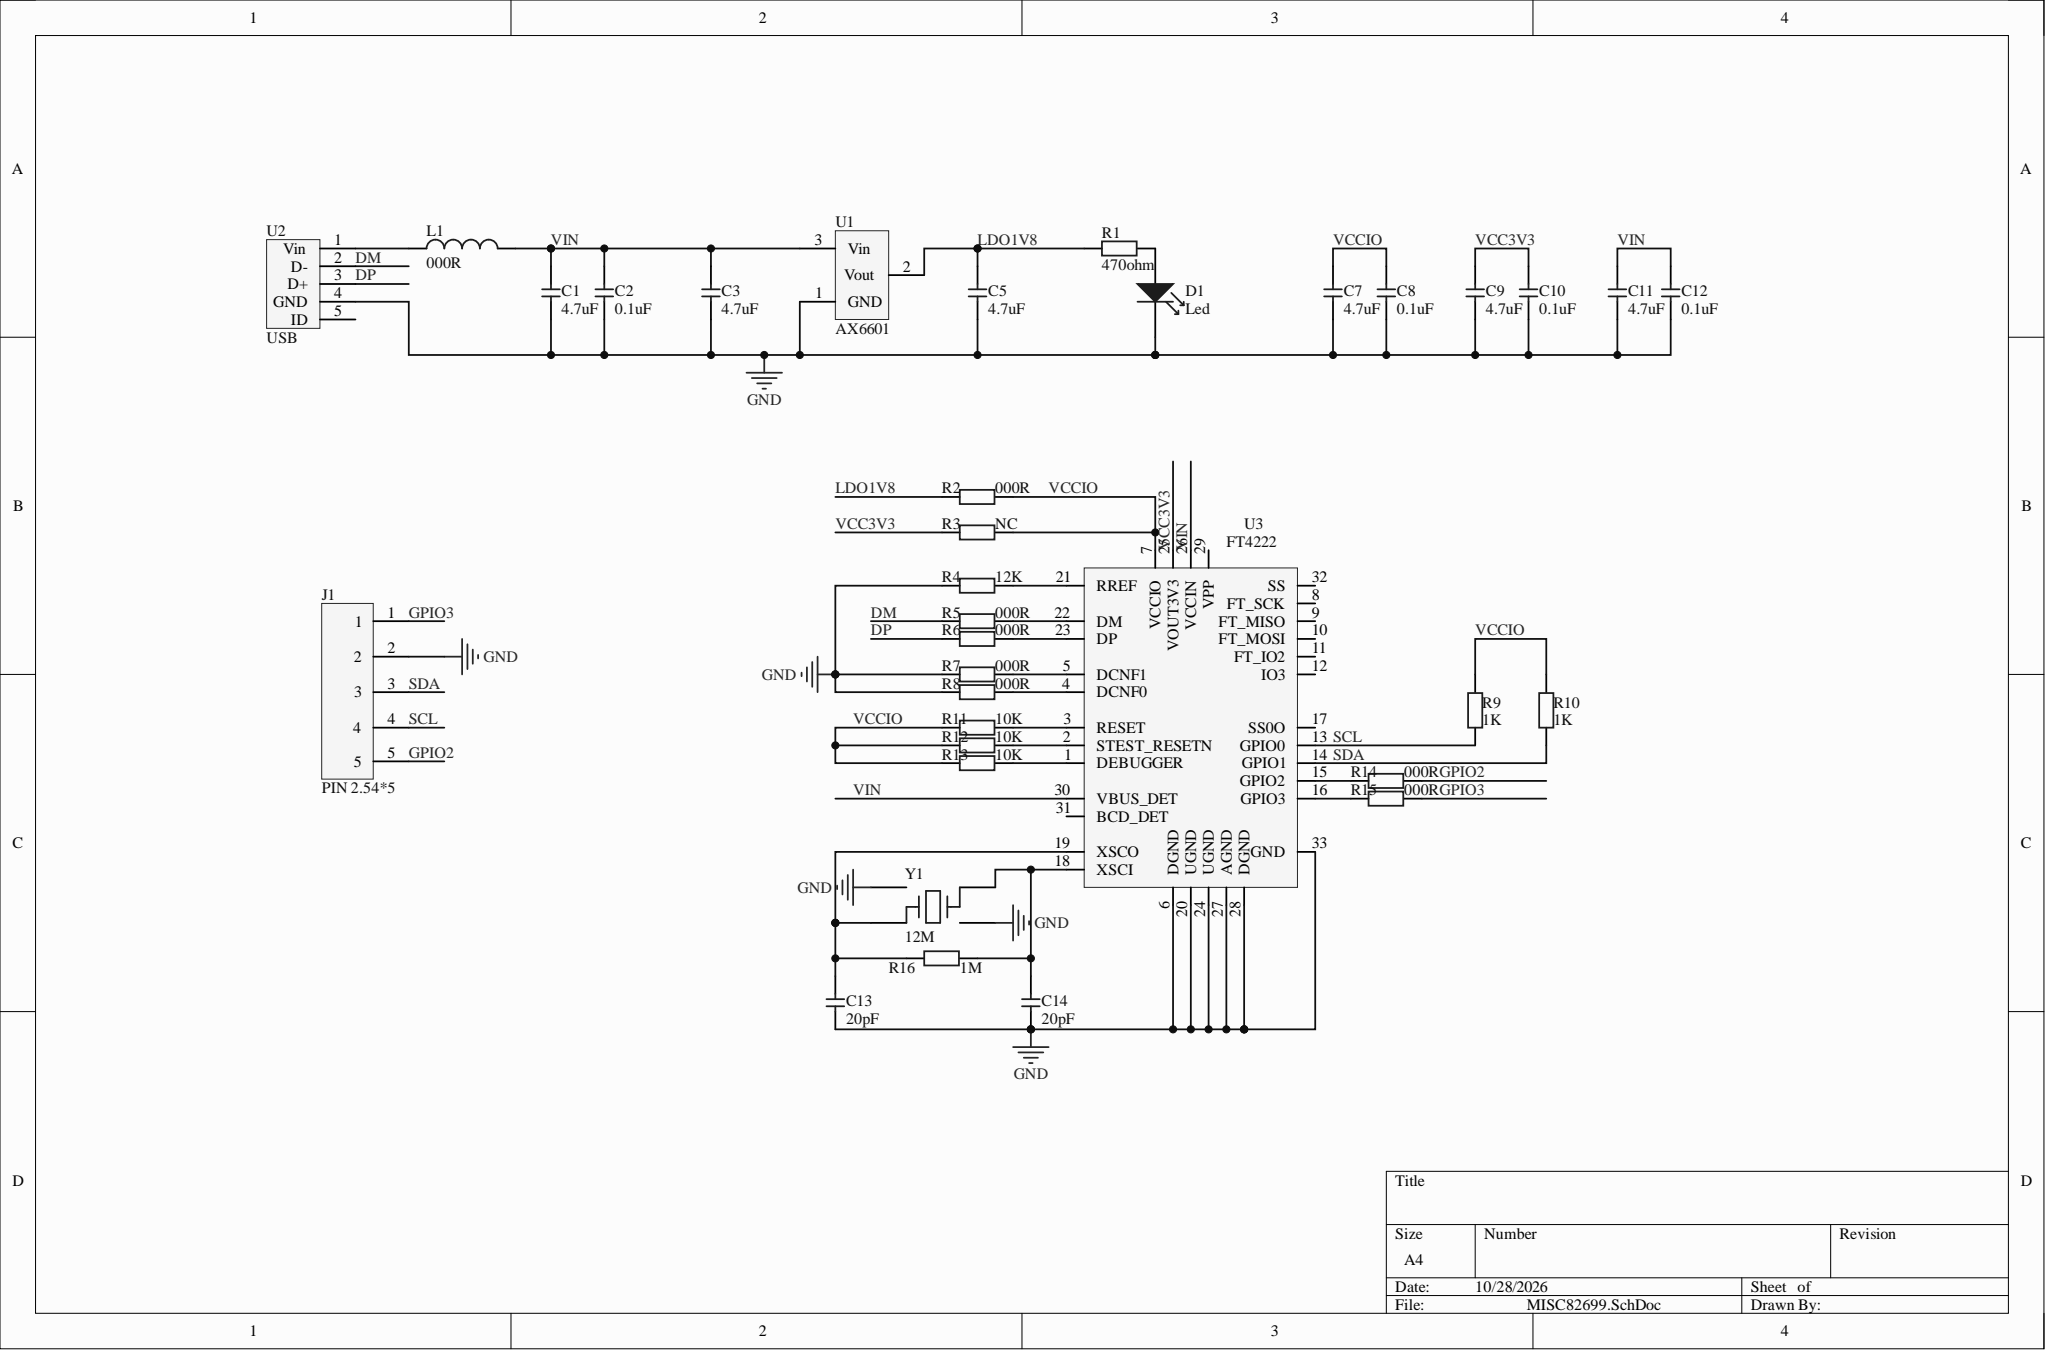Circuit board | Altium Designer | 35 parts | 25 nets
Bill of materials:
Comment,Description,Designator,Footprint,LibRef,Quantity
"4.7uF","","C1, C3, C5, C7, C9, C11","C0402","Cap","6"
"0.1uF","","C2, C8, C10, C12","C0402","Cap","4"
"20pF","","C13, C14","C0402","Cap","2"
"Led","","D1","R0603","Led","1"
"PIN 2.54*5","","J1","DIP2.54*5","PIN_5","1"
"000R","","L1","R0603","Inductor","1"
"470ohm","","R1","R0402","Res","1"
"000R","","R2, R5, R6, R7, R8, R14, R15","R0402","Res","7"
"NC","","R3","R0402","Res","1"
"12K","","R4","R0402","Res","1"
"1K","","R9, R10","R0402","Res","2"
"10K","","R11, R12, R13","R0402","Res","3"
"1M","","R16","R0402","Res","1"
"AX6601","","U1","SOT_23","LDO","1"
"USB","","U2","MicroUSB","Micro USB","1"
"FT4222","","U3","QFN32","FT4222","1"
"12M","","Y1","XTAL_3225","Crystal","1"
Netlist (Protel format):
[
C1
C0402
4.7uF



]
[
C2
C0402
0.1uF



]
[
C3
C0402
4.7uF



]
[
C5
C0402
4.7uF



]
[
C7
C0402
4.7uF



]
[
C8
C0402
0.1uF



]
[
C9
C0402
4.7uF



]
[
C10
C0402
0.1uF



]
[
C11
C0402
4.7uF



]
[
C12
C0402
0.1uF



]
[
C13
C0402
20pF



]
[
C14
C0402
20pF



]
[
D1
R0603
Led



]
[
J1
DIP2.54*5
PIN 2.54*5



]
[
L1
R0603
000R



]
[
R1
R0402
470ohm



]
[
R2
R0402
000R



]
[
R3
R0402
NC



]
[
R4
R0402
12K



]
[
R5
R0402
000R



]
[
R6
R0402
000R



]
[
R7
R0402
000R



]
[
R8
R0402
000R



]
[
R9
R0402
1K



]
[
R10
R0402
1K



]
[
R11
R0402
10K



]
[
R12
R0402
10K



]
[
R13
R0402
10K



]
[
R14
R0402
000R



]
[
R15
R0402
000R



]
[
R16
R0402
1M



]
[
U1
SOT_23
AX6601



]
[
U2
MicroUSB
USB



]
[
U3
QFN32
FT4222



]
[
Y1
XTAL_3225
12M



]
(
VIN
C1-2
C2-2
C3-2
C11-2
C12-2
L1-1
U1-3
U3-26
U3-30
)
(
VCCIO
C7-2
C8-2
R2-2
R3-2
R9-2
R10-2
R11-1
R12-1
R13-1
U3-7
)
(
VCC3V3
C9-2
C10-2
R3-1
U3-25
)
(
SDA
J1-3
R10-1
U3-14
)
(
SCL
J1-4
R9-1
U3-13
)
(
NetR15_1
R15-1
U3-16
)
(
NetR14_1
R14-1
U3-15
)
(
NetR13_2
R13-2
U3-1
)
(
NetR12_2
R12-2
U3-2
)
(
NetR11_2
R11-2
U3-3
)
(
NetR8_2
R8-2
U3-4
)
(
NetR7_2
R7-2
U3-5
)
(
NetR6_2
R6-2
U3-23
)
(
NetR5_2
R5-2
U3-22
)
(
NetR4_2
R4-2
U3-21
)
(
NetL1_2
L1-2
U2-1
)
(
NetD1_2
D1-2
R1-2
)
(
NetC14_2
C14-2
R16-2
U3-18
Y1-3
)
(
NetC13_2
C13-2
R16-1
U3-19
Y1-1
)
(
LDO1V8
C5-2
R1-1
R2-1
U1-2
)
(
GPIO3
J1-1
R15-2
)
(
GPIO2
J1-5
R14-2
)
(
GND
C1-1
C2-1
C3-1
C5-1
C7-1
C8-1
C9-1
C10-1
C11-1
C12-1
C13-1
C14-1
D1-1
J1-2
R4-1
R7-1
R8-1
U1-1
U2-4
U3-6
U3-20
U3-24
U3-27
U3-28
U3-33
Y1-2
Y1-4
)
(
DP
R6-1
U2-3
)
(
DM
R5-1
U2-2
)